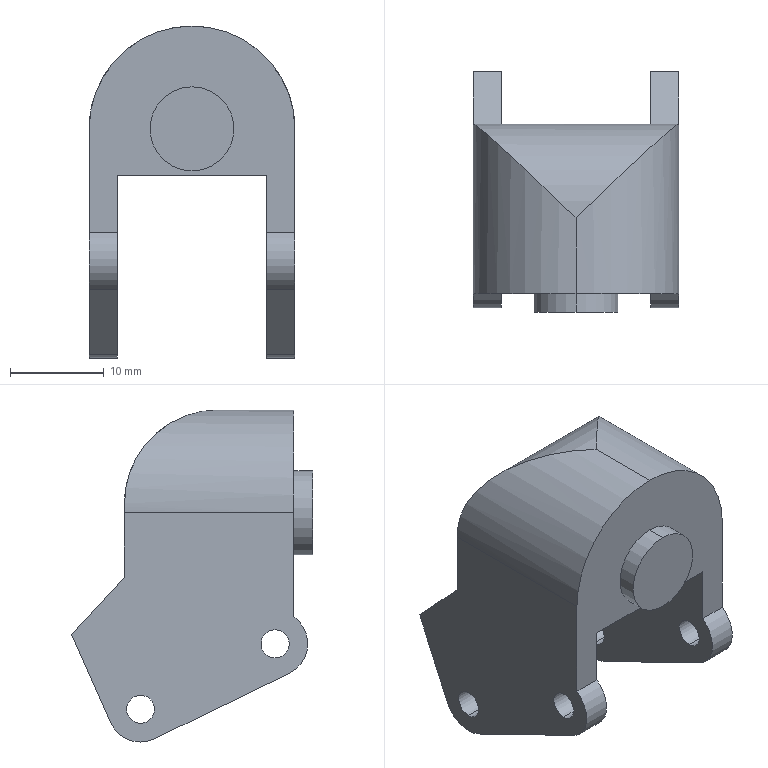Part | STEP file | Deraillieur Bracket End | 1 solid | 31 faces | box 22 x 25.773 x 35.5 mm | volume 7338 mm3 | cylinder 17 | plane 14 | commonest cylinder face diameters 3 x8 7 x4 9 x2 22 x2 20 x1